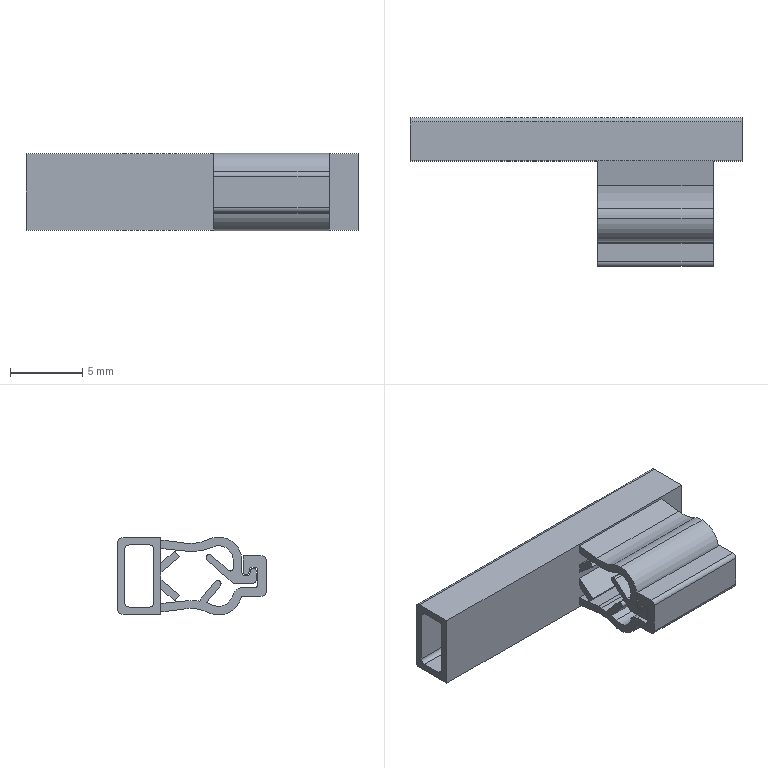Part | SolidWorks | features BaseBody 1 | 1 solid | 81 faces | box 23 x 10.3 x 5.4 mm | volume 293.788 mm3 | plane 45 | cylinder 36 | commonest cylinder face diameters 0.6 x9 0.4 x8 0.45 x4 6.82 x4 2 x3 3.2 x3